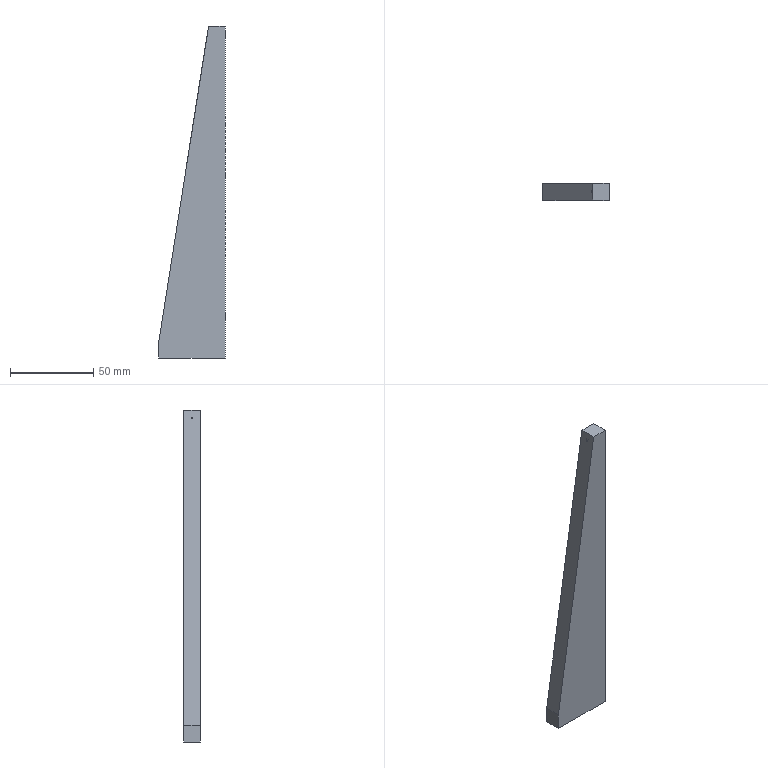Part | SolidWorks | features BaseBody 1 | 1 solid | 27 faces | box 40 x 10 x 200 mm | volume 51054 mm3 | cylinder 10 | cone 10 | plane 7 | commonest cylinder face diameters 3.3 x10
STEP:
#1=CARTESIAN_POINT('',(9.9,0.,96.65));
#2=VERTEX_POINT('',#1);
#3=CARTESIAN_POINT('',(20.,0.,96.65));
#4=VERTEX_POINT('',#3);
#5=CARTESIAN_POINT('',(20.,0.,96.65));
#6=DIRECTION('',(1.,0.,0.));
#7=VECTOR('',#6,1000.);
#8=LINE('',#5,#7);
#9=EDGE_CURVE('',#2,#4,#8,.T.);
#10=ORIENTED_EDGE('',*,*,#9,.F.);
#11=CARTESIAN_POINT('',(9.9,0.,93.35));
#12=VERTEX_POINT('',#11);
#13=CARTESIAN_POINT('',(9.9,0.,95.));
#14=DIRECTION('',(1.,0.,0.));
#15=DIRECTION('',(0.,0.,-1.));
#16=AXIS2_PLACEMENT_3D('',#13,#14,#15);
#17=CIRCLE('',#16,1.65);
#18=EDGE_CURVE('',#12,#2,#17,.T.);
#19=ORIENTED_EDGE('',*,*,#18,.F.);
#20=CARTESIAN_POINT('',(20.,0.,93.35));
#21=VERTEX_POINT('',#20);
#22=CARTESIAN_POINT('',(20.,0.,93.35));
#23=DIRECTION('',(1.,0.,0.));
#24=VECTOR('',#23,1000.);
#25=LINE('',#22,#24);
#26=EDGE_CURVE('',#12,#21,#25,.T.);
#27=ORIENTED_EDGE('',*,*,#26,.T.);
#28=CARTESIAN_POINT('',(20.,0.,95.));
#29=DIRECTION('',(1.,0.,0.));
#30=DIRECTION('',(0.,0.,-1.));
#31=AXIS2_PLACEMENT_3D('',#28,#29,#30);
#32=CIRCLE('',#31,1.65);
#33=EDGE_CURVE('',#21,#4,#32,.T.);
#34=ORIENTED_EDGE('',*,*,#33,.T.);
#35=EDGE_LOOP('',(#10,#19,#27,#34));
#36=FACE_OUTER_BOUND('',#35,.T.);
#37=CARTESIAN_POINT('',(20.,0.,95.));
#38=DIRECTION('',(1.,0.,0.));
#39=DIRECTION('',(0.,0.,-1.));
#40=AXIS2_PLACEMENT_3D('',#37,#38,#39);
#41=CYLINDRICAL_SURFACE('',#40,1.65);
#42=ADVANCED_FACE('',(#36),#41,.F.);
#43=CARTESIAN_POINT('',(9.318,0.,95.682));
#44=VERTEX_POINT('',#43);
#45=CARTESIAN_POINT('',(9.9,0.,96.65));
#46=DIRECTION('',(0.515,0.,0.8572));
#47=VECTOR('',#46,1000.);
#48=LINE('',#45,#47);
#49=EDGE_CURVE('',#44,#2,#48,.T.);
#50=ORIENTED_EDGE('',*,*,#49,.F.);
#51=CARTESIAN_POINT('',(9.148,0.,94.602));
#52=VERTEX_POINT('',#51);
#53=CARTESIAN_POINT('',(9.148,0.,94.602));
#54=CARTESIAN_POINT('',(9.148,1.042,94.602));
#55=CARTESIAN_POINT('',(9.318,1.042,95.682));
#56=CARTESIAN_POINT('',(9.318,0.,95.682));
#57=(BOUNDED_CURVE()B_SPLINE_CURVE(3,(#53,#54,#55,#56),.UNSPECIFIED.,.F.,.F.)B_SPLINE_CURVE_WITH_KNOTS((4,4),(3.142,6.283),.UNSPECIFIED.)CURVE()GEOMETRIC_REPRESENTATION_ITEM()RATIONAL_B_SPLINE_CURVE((1.,0.3333,0.3333,1.))REPRESENTATION_ITEM(''));
#58=EDGE_CURVE('',#52,#44,#57,.T.);
#59=ORIENTED_EDGE('',*,*,#58,.F.);
#60=CARTESIAN_POINT('',(9.9,0.,93.35));
#61=DIRECTION('',(0.515,0.,-0.8572));
#62=VECTOR('',#61,1000.);
#63=LINE('',#60,#62);
#64=EDGE_CURVE('',#52,#12,#63,.T.);
#65=ORIENTED_EDGE('',*,*,#64,.T.);
#66=ORIENTED_EDGE('',*,*,#18,.T.);
#67=EDGE_LOOP('',(#50,#59,#65,#66));
#68=FACE_OUTER_BOUND('',#67,.T.);
#69=CARTESIAN_POINT('',(9.9,0.,95.));
#70=DIRECTION('',(1.,0.,0.));
#71=DIRECTION('',(0.,0.,-1.));
#72=AXIS2_PLACEMENT_3D('',#69,#70,#71);
#73=CONICAL_SURFACE('',#72,1.65,1.03);
#74=ADVANCED_FACE('',(#68),#73,.F.);
#75=CARTESIAN_POINT('',(9.9,0.,11.65));
#76=VERTEX_POINT('',#75);
#77=CARTESIAN_POINT('',(20.,0.,11.65));
#78=VERTEX_POINT('',#77);
#79=CARTESIAN_POINT('',(20.,0.,11.65));
#80=DIRECTION('',(1.,0.,0.));
#81=VECTOR('',#80,1000.);
#82=LINE('',#79,#81);
#83=EDGE_CURVE('',#76,#78,#82,.T.);
#84=ORIENTED_EDGE('',*,*,#83,.F.);
#85=CARTESIAN_POINT('',(9.9,0.,8.35));
#86=VERTEX_POINT('',#85);
#87=CARTESIAN_POINT('',(9.9,0.,10.));
#88=DIRECTION('',(1.,0.,0.));
#89=DIRECTION('',(0.,0.,-1.));
#90=AXIS2_PLACEMENT_3D('',#87,#88,#89);
#91=CIRCLE('',#90,1.65);
#92=EDGE_CURVE('',#86,#76,#91,.T.);
#93=ORIENTED_EDGE('',*,*,#92,.F.);
#94=CARTESIAN_POINT('',(20.,0.,8.35));
#95=VERTEX_POINT('',#94);
#96=CARTESIAN_POINT('',(20.,0.,8.35));
#97=DIRECTION('',(1.,0.,0.));
#98=VECTOR('',#97,1000.);
#99=LINE('',#96,#98);
#100=EDGE_CURVE('',#86,#95,#99,.T.);
#101=ORIENTED_EDGE('',*,*,#100,.T.);
#102=CARTESIAN_POINT('',(20.,0.,10.));
#103=DIRECTION('',(1.,0.,0.));
#104=DIRECTION('',(0.,0.,-1.));
#105=AXIS2_PLACEMENT_3D('',#102,#103,#104);
#106=CIRCLE('',#105,1.65);
#107=EDGE_CURVE('',#95,#78,#106,.T.);
#108=ORIENTED_EDGE('',*,*,#107,.T.);
#109=EDGE_LOOP('',(#84,#93,#101,#108));
#110=FACE_OUTER_BOUND('',#109,.T.);
#111=CARTESIAN_POINT('',(20.,0.,10.));
#112=DIRECTION('',(1.,0.,0.));
#113=DIRECTION('',(0.,0.,-1.));
#114=AXIS2_PLACEMENT_3D('',#111,#112,#113);
#115=CYLINDRICAL_SURFACE('',#114,1.65);
#116=ADVANCED_FACE('',(#110),#115,.F.);
#117=CARTESIAN_POINT('',(8.909,0.,10.));
#118=VERTEX_POINT('',#117);
#119=CARTESIAN_POINT('',(9.9,0.,11.65));
#120=DIRECTION('',(0.515,0.,0.8572));
#121=VECTOR('',#120,1000.);
#122=LINE('',#119,#121);
#123=EDGE_CURVE('',#118,#76,#122,.T.);
#124=ORIENTED_EDGE('',*,*,#123,.F.);
#125=CARTESIAN_POINT('',(9.9,0.,8.35));
#126=DIRECTION('',(0.515,0.,-0.8572));
#127=VECTOR('',#126,1000.);
#128=LINE('',#125,#127);
#129=EDGE_CURVE('',#118,#86,#128,.T.);
#130=ORIENTED_EDGE('',*,*,#129,.T.);
#131=ORIENTED_EDGE('',*,*,#92,.T.);
#132=EDGE_LOOP('',(#124,#130,#131));
#133=FACE_OUTER_BOUND('',#132,.T.);
#134=CARTESIAN_POINT('',(9.9,0.,10.));
#135=DIRECTION('',(1.,0.,0.));
#136=DIRECTION('',(0.,0.,-1.));
#137=AXIS2_PLACEMENT_3D('',#134,#135,#136);
#138=CONICAL_SURFACE('',#137,1.65,1.03);
#139=ADVANCED_FACE('',(#133),#138,.F.);
#140=CARTESIAN_POINT('',(9.9,0.,-73.35));
#141=VERTEX_POINT('',#140);
#142=CARTESIAN_POINT('',(20.,0.,-73.35));
#143=VERTEX_POINT('',#142);
#144=CARTESIAN_POINT('',(20.,0.,-73.35));
#145=DIRECTION('',(1.,0.,0.));
#146=VECTOR('',#145,1000.);
#147=LINE('',#144,#146);
#148=EDGE_CURVE('',#141,#143,#147,.T.);
#149=ORIENTED_EDGE('',*,*,#148,.F.);
#150=CARTESIAN_POINT('',(9.9,0.,-76.65));
#151=VERTEX_POINT('',#150);
#152=CARTESIAN_POINT('',(9.9,0.,-75.));
#153=DIRECTION('',(1.,0.,0.));
#154=DIRECTION('',(0.,0.,-1.));
#155=AXIS2_PLACEMENT_3D('',#152,#153,#154);
#156=CIRCLE('',#155,1.65);
#157=EDGE_CURVE('',#151,#141,#156,.T.);
#158=ORIENTED_EDGE('',*,*,#157,.F.);
#159=CARTESIAN_POINT('',(20.,0.,-76.65));
#160=VERTEX_POINT('',#159);
#161=CARTESIAN_POINT('',(20.,0.,-76.65));
#162=DIRECTION('',(1.,0.,0.));
#163=VECTOR('',#162,1000.);
#164=LINE('',#161,#163);
#165=EDGE_CURVE('',#151,#160,#164,.T.);
#166=ORIENTED_EDGE('',*,*,#165,.T.);
#167=CARTESIAN_POINT('',(20.,0.,-75.));
#168=DIRECTION('',(1.,0.,0.));
#169=DIRECTION('',(0.,0.,-1.));
#170=AXIS2_PLACEMENT_3D('',#167,#168,#169);
#171=CIRCLE('',#170,1.65);
#172=EDGE_CURVE('',#160,#143,#171,.T.);
#173=ORIENTED_EDGE('',*,*,#172,.T.);
#174=EDGE_LOOP('',(#149,#158,#166,#173));
#175=FACE_OUTER_BOUND('',#174,.T.);
#176=CARTESIAN_POINT('',(20.,0.,-75.));
#177=DIRECTION('',(1.,0.,0.));
#178=DIRECTION('',(0.,0.,-1.));
#179=AXIS2_PLACEMENT_3D('',#176,#177,#178);
#180=CYLINDRICAL_SURFACE('',#179,1.65);
#181=ADVANCED_FACE('',(#175),#180,.F.);
#182=CARTESIAN_POINT('',(8.909,0.,-75.));
#183=VERTEX_POINT('',#182);
#184=CARTESIAN_POINT('',(9.9,0.,-73.35));
#185=DIRECTION('',(0.515,0.,0.8572));
#186=VECTOR('',#185,1000.);
#187=LINE('',#184,#186);
#188=EDGE_CURVE('',#183,#141,#187,.T.);
#189=ORIENTED_EDGE('',*,*,#188,.F.);
#190=CARTESIAN_POINT('',(9.9,0.,-76.65));
#191=DIRECTION('',(0.515,0.,-0.8572));
#192=VECTOR('',#191,1000.);
#193=LINE('',#190,#192);
#194=EDGE_CURVE('',#183,#151,#193,.T.);
#195=ORIENTED_EDGE('',*,*,#194,.T.);
#196=ORIENTED_EDGE('',*,*,#157,.T.);
#197=EDGE_LOOP('',(#189,#195,#196));
#198=FACE_OUTER_BOUND('',#197,.T.);
#199=CARTESIAN_POINT('',(9.9,0.,-75.));
#200=DIRECTION('',(1.,0.,0.));
#201=DIRECTION('',(0.,0.,-1.));
#202=AXIS2_PLACEMENT_3D('',#199,#200,#201);
#203=CONICAL_SURFACE('',#202,1.65,1.03);
#204=ADVANCED_FACE('',(#198),#203,.F.);
#205=CARTESIAN_POINT('',(-13.35,0.,-89.9));
#206=VERTEX_POINT('',#205);
#207=CARTESIAN_POINT('',(-13.35,0.,-100.));
#208=VERTEX_POINT('',#207);
#209=CARTESIAN_POINT('',(-13.35,0.,-100.));
#210=DIRECTION('',(0.,0.,-1.));
#211=VECTOR('',#210,1000.);
#212=LINE('',#209,#211);
#213=EDGE_CURVE('',#206,#208,#212,.T.);
#214=ORIENTED_EDGE('',*,*,#213,.F.);
#215=CARTESIAN_POINT('',(-16.65,0.,-89.9));
#216=VERTEX_POINT('',#215);
#217=CARTESIAN_POINT('',(-15.,0.,-89.9));
#218=DIRECTION('',(0.,0.,-1.));
#219=DIRECTION('',(-1.,0.,0.));
#220=AXIS2_PLACEMENT_3D('',#217,#218,#219);
#221=CIRCLE('',#220,1.65);
#222=EDGE_CURVE('',#216,#206,#221,.T.);
#223=ORIENTED_EDGE('',*,*,#222,.F.);
#224=CARTESIAN_POINT('',(-16.65,0.,-100.));
#225=VERTEX_POINT('',#224);
#226=CARTESIAN_POINT('',(-16.65,0.,-100.));
#227=DIRECTION('',(0.,0.,-1.));
#228=VECTOR('',#227,1000.);
#229=LINE('',#226,#228);
#230=EDGE_CURVE('',#216,#225,#229,.T.);
#231=ORIENTED_EDGE('',*,*,#230,.T.);
#232=CARTESIAN_POINT('',(-15.,0.,-100.));
#233=DIRECTION('',(0.,0.,-1.));
#234=DIRECTION('',(-1.,0.,0.));
#235=AXIS2_PLACEMENT_3D('',#232,#233,#234);
#236=CIRCLE('',#235,1.65);
#237=EDGE_CURVE('',#225,#208,#236,.T.);
#238=ORIENTED_EDGE('',*,*,#237,.T.);
#239=EDGE_LOOP('',(#214,#223,#231,#238));
#240=FACE_OUTER_BOUND('',#239,.T.);
#241=CARTESIAN_POINT('',(-15.,0.,-100.));
#242=DIRECTION('',(0.,0.,-1.));
#243=DIRECTION('',(-1.,0.,0.));
#244=AXIS2_PLACEMENT_3D('',#241,#242,#243);
#245=CYLINDRICAL_SURFACE('',#244,1.65);
#246=ADVANCED_FACE('',(#240),#245,.F.);
#247=CARTESIAN_POINT('',(-15.,0.,-88.909));
#248=VERTEX_POINT('',#247);
#249=CARTESIAN_POINT('',(-13.35,0.,-89.9));
#250=DIRECTION('',(0.8572,0.,-0.515));
#251=VECTOR('',#250,1000.);
#252=LINE('',#249,#251);
#253=EDGE_CURVE('',#248,#206,#252,.T.);
#254=ORIENTED_EDGE('',*,*,#253,.F.);
#255=CARTESIAN_POINT('',(-16.65,0.,-89.9));
#256=DIRECTION('',(-0.8572,0.,-0.515));
#257=VECTOR('',#256,1000.);
#258=LINE('',#255,#257);
#259=EDGE_CURVE('',#248,#216,#258,.T.);
#260=ORIENTED_EDGE('',*,*,#259,.T.);
#261=ORIENTED_EDGE('',*,*,#222,.T.);
#262=EDGE_LOOP('',(#254,#260,#261));
#263=FACE_OUTER_BOUND('',#262,.T.);
#264=CARTESIAN_POINT('',(-15.,0.,-89.9));
#265=DIRECTION('',(0.,0.,-1.));
#266=DIRECTION('',(-1.,0.,0.));
#267=AXIS2_PLACEMENT_3D('',#264,#265,#266);
#268=CONICAL_SURFACE('',#267,1.65,1.03);
#269=ADVANCED_FACE('',(#263),#268,.F.);
#270=CARTESIAN_POINT('',(11.65,0.,-89.9));
#271=VERTEX_POINT('',#270);
#272=CARTESIAN_POINT('',(11.65,0.,-100.));
#273=VERTEX_POINT('',#272);
#274=CARTESIAN_POINT('',(11.65,0.,-100.));
#275=DIRECTION('',(0.,0.,-1.));
#276=VECTOR('',#275,1000.);
#277=LINE('',#274,#276);
#278=EDGE_CURVE('',#271,#273,#277,.T.);
#279=ORIENTED_EDGE('',*,*,#278,.F.);
#280=CARTESIAN_POINT('',(8.35,0.,-89.9));
#281=VERTEX_POINT('',#280);
#282=CARTESIAN_POINT('',(10.,0.,-89.9));
#283=DIRECTION('',(0.,0.,-1.));
#284=DIRECTION('',(-1.,0.,0.));
#285=AXIS2_PLACEMENT_3D('',#282,#283,#284);
#286=CIRCLE('',#285,1.65);
#287=EDGE_CURVE('',#281,#271,#286,.T.);
#288=ORIENTED_EDGE('',*,*,#287,.F.);
#289=CARTESIAN_POINT('',(8.35,0.,-100.));
#290=VERTEX_POINT('',#289);
#291=CARTESIAN_POINT('',(8.35,0.,-100.));
#292=DIRECTION('',(0.,0.,-1.));
#293=VECTOR('',#292,1000.);
#294=LINE('',#291,#293);
#295=EDGE_CURVE('',#281,#290,#294,.T.);
#296=ORIENTED_EDGE('',*,*,#295,.T.);
#297=CARTESIAN_POINT('',(10.,0.,-100.));
#298=DIRECTION('',(0.,0.,-1.));
#299=DIRECTION('',(-1.,0.,0.));
#300=AXIS2_PLACEMENT_3D('',#297,#298,#299);
#301=CIRCLE('',#300,1.65);
#302=EDGE_CURVE('',#290,#273,#301,.T.);
#303=ORIENTED_EDGE('',*,*,#302,.T.);
#304=EDGE_LOOP('',(#279,#288,#296,#303));
#305=FACE_OUTER_BOUND('',#304,.T.);
#306=CARTESIAN_POINT('',(10.,0.,-100.));
#307=DIRECTION('',(0.,0.,-1.));
#308=DIRECTION('',(-1.,0.,0.));
#309=AXIS2_PLACEMENT_3D('',#306,#307,#308);
#310=CYLINDRICAL_SURFACE('',#309,1.65);
#311=ADVANCED_FACE('',(#305),#310,.F.);
#312=CARTESIAN_POINT('',(10.,0.,-88.909));
#313=VERTEX_POINT('',#312);
#314=CARTESIAN_POINT('',(11.65,0.,-89.9));
#315=DIRECTION('',(0.8572,0.,-0.515));
#316=VECTOR('',#315,1000.);
#317=LINE('',#314,#316);
#318=EDGE_CURVE('',#313,#271,#317,.T.);
#319=ORIENTED_EDGE('',*,*,#318,.F.);
#320=CARTESIAN_POINT('',(8.35,0.,-89.9));
#321=DIRECTION('',(-0.8572,0.,-0.515));
#322=VECTOR('',#321,1000.);
#323=LINE('',#320,#322);
#324=EDGE_CURVE('',#313,#281,#323,.T.);
#325=ORIENTED_EDGE('',*,*,#324,.T.);
#326=ORIENTED_EDGE('',*,*,#287,.T.);
#327=EDGE_LOOP('',(#319,#325,#326));
#328=FACE_OUTER_BOUND('',#327,.T.);
#329=CARTESIAN_POINT('',(10.,0.,-89.9));
#330=DIRECTION('',(0.,0.,-1.));
#331=DIRECTION('',(-1.,0.,0.));
#332=AXIS2_PLACEMENT_3D('',#329,#330,#331);
#333=CONICAL_SURFACE('',#332,1.65,1.03);
#334=ADVANCED_FACE('',(#328),#333,.F.);
#335=ORIENTED_EDGE('',*,*,#58,.T.);
#336=CARTESIAN_POINT('',(9.318,0.,95.682));
#337=CARTESIAN_POINT('',(9.318,-1.042,95.682));
#338=CARTESIAN_POINT('',(9.148,-1.042,94.602));
#339=CARTESIAN_POINT('',(9.148,0.,94.602));
#340=(BOUNDED_CURVE()B_SPLINE_CURVE(3,(#336,#337,#338,#339),.UNSPECIFIED.,.F.,.F.)B_SPLINE_CURVE_WITH_KNOTS((4,4),(0.,3.142),.UNSPECIFIED.)CURVE()GEOMETRIC_REPRESENTATION_ITEM()RATIONAL_B_SPLINE_CURVE((1.,0.3333,0.3333,1.))REPRESENTATION_ITEM(''));
#341=EDGE_CURVE('',#44,#52,#340,.T.);
#342=ORIENTED_EDGE('',*,*,#341,.T.);
#343=EDGE_LOOP('',(#335,#342));
#344=FACE_BOUND('',#343,.T.);
#345=CARTESIAN_POINT('',(10.,-5.,100.));
#346=VERTEX_POINT('',#345);
#347=CARTESIAN_POINT('',(10.,5.,100.));
#348=VERTEX_POINT('',#347);
#349=CARTESIAN_POINT('',(10.,-197.354,100.));
#350=DIRECTION('',(0.,1.,0.));
#351=VECTOR('',#350,1000.);
#352=LINE('',#349,#351);
#353=EDGE_CURVE('',#346,#348,#352,.T.);
#354=ORIENTED_EDGE('',*,*,#353,.T.);
#355=CARTESIAN_POINT('',(-20.,5.,-90.));
#356=VERTEX_POINT('',#355);
#357=CARTESIAN_POINT('',(10.,5.,100.));
#358=DIRECTION('',(-0.156,0.,-0.9878));
#359=VECTOR('',#358,1000.);
#360=LINE('',#357,#359);
#361=EDGE_CURVE('',#348,#356,#360,.T.);
#362=ORIENTED_EDGE('',*,*,#361,.T.);
#363=CARTESIAN_POINT('',(-20.,-5.,-90.));
#364=VERTEX_POINT('',#363);
#365=CARTESIAN_POINT('',(-20.,-197.354,-90.));
#366=DIRECTION('',(0.,1.,0.));
#367=VECTOR('',#366,1000.);
#368=LINE('',#365,#367);
#369=EDGE_CURVE('',#364,#356,#368,.T.);
#370=ORIENTED_EDGE('',*,*,#369,.F.);
#371=CARTESIAN_POINT('',(10.,-5.,100.));
#372=DIRECTION('',(-0.156,0.,-0.9878));
#373=VECTOR('',#372,1000.);
#374=LINE('',#371,#373);
#375=EDGE_CURVE('',#346,#364,#374,.T.);
#376=ORIENTED_EDGE('',*,*,#375,.F.);
#377=EDGE_LOOP('',(#354,#362,#370,#376));
#378=FACE_OUTER_BOUND('',#377,.T.);
#379=CARTESIAN_POINT('',(10.,-197.354,100.));
#380=DIRECTION('',(0.9878,0.,-0.156));
#381=DIRECTION('',(0.,-1.,0.));
#382=AXIS2_PLACEMENT_3D('',#379,#380,#381);
#383=PLANE('',#382);
#384=ADVANCED_FACE('',(#344,#378),#383,.F.);
#385=ORIENTED_EDGE('',*,*,#375,.T.);
#386=CARTESIAN_POINT('',(-20.,-5.,-100.));
#387=VERTEX_POINT('',#386);
#388=CARTESIAN_POINT('',(-20.,-5.,100.));
#389=DIRECTION('',(0.,0.,1.));
#390=VECTOR('',#389,1000.);
#391=LINE('',#388,#390);
#392=EDGE_CURVE('',#387,#364,#391,.T.);
#393=ORIENTED_EDGE('',*,*,#392,.F.);
#394=CARTESIAN_POINT('',(20.,-5.,-100.));
#395=VERTEX_POINT('',#394);
#396=CARTESIAN_POINT('',(-20.,-5.,-100.));
#397=DIRECTION('',(-1.,0.,0.));
#398=VECTOR('',#397,1000.);
#399=LINE('',#396,#398);
#400=EDGE_CURVE('',#395,#387,#399,.T.);
#401=ORIENTED_EDGE('',*,*,#400,.F.);
#402=CARTESIAN_POINT('',(20.,-5.,100.));
#403=VERTEX_POINT('',#402);
#404=CARTESIAN_POINT('',(20.,-5.,100.));
#405=DIRECTION('',(0.,0.,-1.));
#406=VECTOR('',#405,1000.);
#407=LINE('',#404,#406);
#408=EDGE_CURVE('',#403,#395,#407,.T.);
#409=ORIENTED_EDGE('',*,*,#408,.F.);
#410=CARTESIAN_POINT('',(-20.,-5.,100.));
#411=DIRECTION('',(1.,0.,0.));
#412=VECTOR('',#411,1000.);
#413=LINE('',#410,#412);
#414=EDGE_CURVE('',#346,#403,#413,.T.);
#415=ORIENTED_EDGE('',*,*,#414,.F.);
#416=EDGE_LOOP('',(#385,#393,#401,#409,#415));
#417=FACE_OUTER_BOUND('',#416,.T.);
#418=CARTESIAN_POINT('',(0.,-5.,0.));
#419=DIRECTION('',(0.,-1.,0.));
#420=DIRECTION('',(0.,0.,-1.));
#421=AXIS2_PLACEMENT_3D('',#418,#419,#420);
#422=PLANE('',#421);
#423=ADVANCED_FACE('',(#417),#422,.T.);
#424=CARTESIAN_POINT('',(-20.,5.,-100.));
#425=VERTEX_POINT('',#424);
#426=CARTESIAN_POINT('',(-20.,5.,100.));
#427=DIRECTION('',(0.,0.,1.));
#428=VECTOR('',#427,1000.);
#429=LINE('',#426,#428);
#430=EDGE_CURVE('',#425,#356,#429,.T.);
#431=ORIENTED_EDGE('',*,*,#430,.T.);
#432=ORIENTED_EDGE('',*,*,#361,.F.);
#433=CARTESIAN_POINT('',(20.,5.,100.));
#434=VERTEX_POINT('',#433);
#435=CARTESIAN_POINT('',(-20.,5.,100.));
#436=DIRECTION('',(1.,0.,0.));
#437=VECTOR('',#436,1000.);
#438=LINE('',#435,#437);
#439=EDGE_CURVE('',#348,#434,#438,.T.);
#440=ORIENTED_EDGE('',*,*,#439,.T.);
#441=CARTESIAN_POINT('',(20.,5.,-100.));
#442=VERTEX_POINT('',#441);
#443=CARTESIAN_POINT('',(20.,5.,100.));
#444=DIRECTION('',(0.,0.,-1.));
#445=VECTOR('',#444,1000.);
#446=LINE('',#443,#445);
#447=EDGE_CURVE('',#434,#442,#446,.T.);
#448=ORIENTED_EDGE('',*,*,#447,.T.);
#449=CARTESIAN_POINT('',(-20.,5.,-100.));
#450=DIRECTION('',(-1.,0.,0.));
#451=VECTOR('',#450,1000.);
#452=LINE('',#449,#451);
#453=EDGE_CURVE('',#442,#425,#452,.T.);
#454=ORIENTED_EDGE('',*,*,#453,.T.);
#455=EDGE_LOOP('',(#431,#432,#440,#448,#454));
#456=FACE_OUTER_BOUND('',#455,.T.);
#457=CARTESIAN_POINT('',(0.,5.,0.));
#458=DIRECTION('',(0.,-1.,0.));
#459=DIRECTION('',(0.,0.,-1.));
#460=AXIS2_PLACEMENT_3D('',#457,#458,#459);
#461=PLANE('',#460);
#462=ADVANCED_FACE('',(#456),#461,.F.);
#463=ORIENTED_EDGE('',*,*,#439,.F.);
#464=ORIENTED_EDGE('',*,*,#353,.F.);
#465=ORIENTED_EDGE('',*,*,#414,.T.);
#466=CARTESIAN_POINT('',(20.,5.,100.));
#467=DIRECTION('',(0.,-1.,0.));
#468=VECTOR('',#467,1000.);
#469=LINE('',#466,#468);
#470=EDGE_CURVE('',#434,#403,#469,.T.);
#471=ORIENTED_EDGE('',*,*,#470,.F.);
#472=EDGE_LOOP('',(#463,#464,#465,#471));
#473=FACE_OUTER_BOUND('',#472,.T.);
#474=CARTESIAN_POINT('',(-20.,5.,100.));
#475=DIRECTION('',(0.,0.,-1.));
#476=DIRECTION('',(0.,-1.,0.));
#477=AXIS2_PLACEMENT_3D('',#474,#475,#476);
#478=PLANE('',#477);
#479=ADVANCED_FACE('',(#473),#478,.F.);
#480=ORIENTED_EDGE('',*,*,#392,.T.);
#481=ORIENTED_EDGE('',*,*,#369,.T.);
#482=ORIENTED_EDGE('',*,*,#430,.F.);
#483=CARTESIAN_POINT('',(-20.,5.,-100.));
#484=DIRECTION('',(0.,-1.,0.));
#485=VECTOR('',#484,1000.);
#486=LINE('',#483,#485);
#487=EDGE_CURVE('',#425,#387,#486,.T.);
#488=ORIENTED_EDGE('',*,*,#487,.T.);
#489=EDGE_LOOP('',(#480,#481,#482,#488));
#490=FACE_OUTER_BOUND('',#489,.T.);
#491=CARTESIAN_POINT('',(-20.,5.,100.));
#492=DIRECTION('',(1.,0.,0.));
#493=DIRECTION('',(0.,1.,0.));
#494=AXIS2_PLACEMENT_3D('',#491,#492,#493);
#495=PLANE('',#494);
#496=ADVANCED_FACE('',(#490),#495,.F.);
#497=ORIENTED_EDGE('',*,*,#302,.F.);
#498=CARTESIAN_POINT('',(10.,0.,-100.));
#499=DIRECTION('',(0.,0.,-1.));
#500=DIRECTION('',(-1.,0.,0.));
#501=AXIS2_PLACEMENT_3D('',#498,#499,#500);
#502=CIRCLE('',#501,1.65);
#503=EDGE_CURVE('',#273,#290,#502,.T.);
#504=ORIENTED_EDGE('',*,*,#503,.F.);
#505=EDGE_LOOP('',(#497,#504));
#506=FACE_BOUND('',#505,.T.);
#507=ORIENTED_EDGE('',*,*,#237,.F.);
#508=CARTESIAN_POINT('',(-15.,0.,-100.));
#509=DIRECTION('',(0.,0.,-1.));
#510=DIRECTION('',(-1.,0.,0.));
#511=AXIS2_PLACEMENT_3D('',#508,#509,#510);
#512=CIRCLE('',#511,1.65);
#513=EDGE_CURVE('',#208,#225,#512,.T.);
#514=ORIENTED_EDGE('',*,*,#513,.F.);
#515=EDGE_LOOP('',(#507,#514));
#516=FACE_BOUND('',#515,.T.);
#517=ORIENTED_EDGE('',*,*,#400,.T.);
#518=ORIENTED_EDGE('',*,*,#487,.F.);
#519=ORIENTED_EDGE('',*,*,#453,.F.);
#520=CARTESIAN_POINT('',(20.,5.,-100.));
#521=DIRECTION('',(0.,-1.,0.));
#522=VECTOR('',#521,1000.);
#523=LINE('',#520,#522);
#524=EDGE_CURVE('',#442,#395,#523,.T.);
#525=ORIENTED_EDGE('',*,*,#524,.T.);
#526=EDGE_LOOP('',(#517,#518,#519,#525));
#527=FACE_OUTER_BOUND('',#526,.T.);
#528=CARTESIAN_POINT('',(-20.,5.,-100.));
#529=DIRECTION('',(0.,0.,1.));
#530=DIRECTION('',(1.,0.,0.));
#531=AXIS2_PLACEMENT_3D('',#528,#529,#530);
#532=PLANE('',#531);
#533=ADVANCED_FACE('',(#506,#516,#527),#532,.F.);
#534=ORIENTED_EDGE('',*,*,#172,.F.);
#535=CARTESIAN_POINT('',(20.,0.,-75.));
#536=DIRECTION('',(1.,0.,0.));
#537=DIRECTION('',(0.,0.,-1.));
#538=AXIS2_PLACEMENT_3D('',#535,#536,#537);
#539=CIRCLE('',#538,1.65);
#540=EDGE_CURVE('',#143,#160,#539,.T.);
#541=ORIENTED_EDGE('',*,*,#540,.F.);
#542=EDGE_LOOP('',(#534,#541));
#543=FACE_BOUND('',#542,.T.);
#544=ORIENTED_EDGE('',*,*,#107,.F.);
#545=CARTESIAN_POINT('',(20.,0.,10.));
#546=DIRECTION('',(1.,0.,0.));
#547=DIRECTION('',(0.,0.,-1.));
#548=AXIS2_PLACEMENT_3D('',#545,#546,#547);
#549=CIRCLE('',#548,1.65);
#550=EDGE_CURVE('',#78,#95,#549,.T.);
#551=ORIENTED_EDGE('',*,*,#550,.F.);
#552=EDGE_LOOP('',(#544,#551));
#553=FACE_BOUND('',#552,.T.);
#554=ORIENTED_EDGE('',*,*,#33,.F.);
#555=CARTESIAN_POINT('',(20.,0.,95.));
#556=DIRECTION('',(1.,0.,0.));
#557=DIRECTION('',(0.,0.,-1.));
#558=AXIS2_PLACEMENT_3D('',#555,#556,#557);
#559=CIRCLE('',#558,1.65);
#560=EDGE_CURVE('',#4,#21,#559,.T.);
#561=ORIENTED_EDGE('',*,*,#560,.F.);
#562=EDGE_LOOP('',(#554,#561));
#563=FACE_BOUND('',#562,.T.);
#564=ORIENTED_EDGE('',*,*,#408,.T.);
#565=ORIENTED_EDGE('',*,*,#524,.F.);
#566=ORIENTED_EDGE('',*,*,#447,.F.);
#567=ORIENTED_EDGE('',*,*,#470,.T.);
#568=EDGE_LOOP('',(#564,#565,#566,#567));
#569=FACE_OUTER_BOUND('',#568,.T.);
#570=CARTESIAN_POINT('',(20.,5.,100.));
#571=DIRECTION('',(-1.,0.,0.));
#572=DIRECTION('',(0.,0.,1.));
#573=AXIS2_PLACEMENT_3D('',#570,#571,#572);
#574=PLANE('',#573);
#575=ADVANCED_FACE('',(#543,#553,#563,#569),#574,.F.);
#576=ORIENTED_EDGE('',*,*,#324,.F.);
#577=ORIENTED_EDGE('',*,*,#318,.T.);
#578=CARTESIAN_POINT('',(10.,0.,-89.9));
#579=DIRECTION('',(0.,0.,-1.));
#580=DIRECTION('',(-1.,0.,0.));
#581=AXIS2_PLACEMENT_3D('',#578,#579,#580);
#582=CIRCLE('',#581,1.65);
#583=EDGE_CURVE('',#271,#281,#582,.T.);
#584=ORIENTED_EDGE('',*,*,#583,.T.);
#585=EDGE_LOOP('',(#576,#577,#584));
#586=FACE_OUTER_BOUND('',#585,.T.);
#587=CARTESIAN_POINT('',(10.,0.,-89.9));
#588=DIRECTION('',(0.,0.,-1.));
#589=DIRECTION('',(-1.,0.,0.));
#590=AXIS2_PLACEMENT_3D('',#587,#588,#589);
#591=CONICAL_SURFACE('',#590,1.65,1.03);
#592=ADVANCED_FACE('',(#586),#591,.F.);
#593=ORIENTED_EDGE('',*,*,#583,.F.);
#594=ORIENTED_EDGE('',*,*,#278,.T.);
#595=ORIENTED_EDGE('',*,*,#503,.T.);
#596=ORIENTED_EDGE('',*,*,#295,.F.);
#597=EDGE_LOOP('',(#593,#594,#595,#596));
#598=FACE_OUTER_BOUND('',#597,.T.);
#599=CARTESIAN_POINT('',(10.,0.,-100.));
#600=DIRECTION('',(0.,0.,-1.));
#601=DIRECTION('',(-1.,0.,0.));
#602=AXIS2_PLACEMENT_3D('',#599,#600,#601);
#603=CYLINDRICAL_SURFACE('',#602,1.65);
#604=ADVANCED_FACE('',(#598),#603,.F.);
#605=ORIENTED_EDGE('',*,*,#259,.F.);
#606=ORIENTED_EDGE('',*,*,#253,.T.);
#607=CARTESIAN_POINT('',(-15.,0.,-89.9));
#608=DIRECTION('',(0.,0.,-1.));
#609=DIRECTION('',(-1.,0.,0.));
#610=AXIS2_PLACEMENT_3D('',#607,#608,#609);
#611=CIRCLE('',#610,1.65);
#612=EDGE_CURVE('',#206,#216,#611,.T.);
#613=ORIENTED_EDGE('',*,*,#612,.T.);
#614=EDGE_LOOP('',(#605,#606,#613));
#615=FACE_OUTER_BOUND('',#614,.T.);
#616=CARTESIAN_POINT('',(-15.,0.,-89.9));
#617=DIRECTION('',(0.,0.,-1.));
#618=DIRECTION('',(-1.,0.,0.));
#619=AXIS2_PLACEMENT_3D('',#616,#617,#618);
#620=CONICAL_SURFACE('',#619,1.65,1.03);
#621=ADVANCED_FACE('',(#615),#620,.F.);
#622=ORIENTED_EDGE('',*,*,#612,.F.);
#623=ORIENTED_EDGE('',*,*,#213,.T.);
#624=ORIENTED_EDGE('',*,*,#513,.T.);
#625=ORIENTED_EDGE('',*,*,#230,.F.);
#626=EDGE_LOOP('',(#622,#623,#624,#625));
#627=FACE_OUTER_BOUND('',#626,.T.);
#628=CARTESIAN_POINT('',(-15.,0.,-100.));
#629=DIRECTION('',(0.,0.,-1.));
#630=DIRECTION('',(-1.,0.,0.));
#631=AXIS2_PLACEMENT_3D('',#628,#629,#630);
#632=CYLINDRICAL_SURFACE('',#631,1.65);
#633=ADVANCED_FACE('',(#627),#632,.F.);
#634=ORIENTED_EDGE('',*,*,#194,.F.);
#635=ORIENTED_EDGE('',*,*,#188,.T.);
#636=CARTESIAN_POINT('',(9.9,0.,-75.));
#637=DIRECTION('',(1.,0.,0.));
#638=DIRECTION('',(0.,0.,-1.));
#639=AXIS2_PLACEMENT_3D('',#636,#637,#638);
#640=CIRCLE('',#639,1.65);
#641=EDGE_CURVE('',#141,#151,#640,.T.);
#642=ORIENTED_EDGE('',*,*,#641,.T.);
#643=EDGE_LOOP('',(#634,#635,#642));
#644=FACE_OUTER_BOUND('',#643,.T.);
#645=CARTESIAN_POINT('',(9.9,0.,-75.));
#646=DIRECTION('',(1.,0.,0.));
#647=DIRECTION('',(0.,0.,-1.));
#648=AXIS2_PLACEMENT_3D('',#645,#646,#647);
#649=CONICAL_SURFACE('',#648,1.65,1.03);
#650=ADVANCED_FACE('',(#644),#649,.F.);
#651=ORIENTED_EDGE('',*,*,#641,.F.);
#652=ORIENTED_EDGE('',*,*,#148,.T.);
#653=ORIENTED_EDGE('',*,*,#540,.T.);
#654=ORIENTED_EDGE('',*,*,#165,.F.);
#655=EDGE_LOOP('',(#651,#652,#653,#654));
#656=FACE_OUTER_BOUND('',#655,.T.);
#657=CARTESIAN_POINT('',(20.,0.,-75.));
#658=DIRECTION('',(1.,0.,0.));
#659=DIRECTION('',(0.,0.,-1.));
#660=AXIS2_PLACEMENT_3D('',#657,#658,#659);
#661=CYLINDRICAL_SURFACE('',#660,1.65);
#662=ADVANCED_FACE('',(#656),#661,.F.);
#663=ORIENTED_EDGE('',*,*,#129,.F.);
#664=ORIENTED_EDGE('',*,*,#123,.T.);
#665=CARTESIAN_POINT('',(9.9,0.,10.));
#666=DIRECTION('',(1.,0.,0.));
#667=DIRECTION('',(0.,0.,-1.));
#668=AXIS2_PLACEMENT_3D('',#665,#666,#667);
#669=CIRCLE('',#668,1.65);
#670=EDGE_CURVE('',#76,#86,#669,.T.);
#671=ORIENTED_EDGE('',*,*,#670,.T.);
#672=EDGE_LOOP('',(#663,#664,#671));
#673=FACE_OUTER_BOUND('',#672,.T.);
#674=CARTESIAN_POINT('',(9.9,0.,10.));
#675=DIRECTION('',(1.,0.,0.));
#676=DIRECTION('',(0.,0.,-1.));
#677=AXIS2_PLACEMENT_3D('',#674,#675,#676);
#678=CONICAL_SURFACE('',#677,1.65,1.03);
#679=ADVANCED_FACE('',(#673),#678,.F.);
#680=ORIENTED_EDGE('',*,*,#670,.F.);
#681=ORIENTED_EDGE('',*,*,#83,.T.);
#682=ORIENTED_EDGE('',*,*,#550,.T.);
#683=ORIENTED_EDGE('',*,*,#100,.F.);
#684=EDGE_LOOP('',(#680,#681,#682,#683));
#685=FACE_OUTER_BOUND('',#684,.T.);
#686=CARTESIAN_POINT('',(20.,0.,10.));
#687=DIRECTION('',(1.,0.,0.));
#688=DIRECTION('',(0.,0.,-1.));
#689=AXIS2_PLACEMENT_3D('',#686,#687,#688);
#690=CYLINDRICAL_SURFACE('',#689,1.65);
#691=ADVANCED_FACE('',(#685),#690,.F.);
#692=ORIENTED_EDGE('',*,*,#341,.F.);
#693=ORIENTED_EDGE('',*,*,#49,.T.);
#694=CARTESIAN_POINT('',(9.9,0.,95.));
#695=DIRECTION('',(1.,0.,0.));
#696=DIRECTION('',(0.,0.,-1.));
#697=AXIS2_PLACEMENT_3D('',#694,#695,#696);
#698=CIRCLE('',#697,1.65);
#699=EDGE_CURVE('',#2,#12,#698,.T.);
#700=ORIENTED_EDGE('',*,*,#699,.T.);
#701=ORIENTED_EDGE('',*,*,#64,.F.);
#702=EDGE_LOOP('',(#692,#693,#700,#701));
#703=FACE_OUTER_BOUND('',#702,.T.);
#704=CARTESIAN_POINT('',(9.9,0.,95.));
#705=DIRECTION('',(1.,0.,0.));
#706=DIRECTION('',(0.,0.,-1.));
#707=AXIS2_PLACEMENT_3D('',#704,#705,#706);
#708=CONICAL_SURFACE('',#707,1.65,1.03);
#709=ADVANCED_FACE('',(#703),#708,.F.);
#710=ORIENTED_EDGE('',*,*,#699,.F.);
#711=ORIENTED_EDGE('',*,*,#9,.T.);
#712=ORIENTED_EDGE('',*,*,#560,.T.);
#713=ORIENTED_EDGE('',*,*,#26,.F.);
#714=EDGE_LOOP('',(#710,#711,#712,#713));
#715=FACE_OUTER_BOUND('',#714,.T.);
#716=CARTESIAN_POINT('',(20.,0.,95.));
#717=DIRECTION('',(1.,0.,0.));
#718=DIRECTION('',(0.,0.,-1.));
#719=AXIS2_PLACEMENT_3D('',#716,#717,#718);
#720=CYLINDRICAL_SURFACE('',#719,1.65);
#721=ADVANCED_FACE('',(#715),#720,.F.);
#722=CLOSED_SHELL('',(#42,#74,#116,#139,#181,#204,#246,#269,#311,#334,#384,#423,#462,#479,#496,#533,#575,#592,#604,#621,#633,#650,#662,#679,#691,#709,#721));
#723=MANIFOLD_SOLID_BREP('',#722);
#724=CARTESIAN_POINT('',(0.,0.,0.));
#725=DIRECTION('',(0.,0.,1.));
#726=DIRECTION('',(1.,0.,0.));
#727=AXIS2_PLACEMENT_3D('',#724,#725,#726);
#728=(LENGTH_UNIT()NAMED_UNIT(*)SI_UNIT(.MILLI.,.METRE.));
#729=UNCERTAINTY_MEASURE_WITH_UNIT(LENGTH_MEASURE(0.00001),#728,'','');
#730=(NAMED_UNIT(*)PLANE_ANGLE_UNIT()SI_UNIT($,.RADIAN.));
#731=(NAMED_UNIT(*)SI_UNIT($,.STERADIAN.)SOLID_ANGLE_UNIT());
#732=(GEOMETRIC_REPRESENTATION_CONTEXT(3)GLOBAL_UNCERTAINTY_ASSIGNED_CONTEXT((#729))GLOBAL_UNIT_ASSIGNED_CONTEXT((#728,#730,#731))REPRESENTATION_CONTEXT('',''));
#733=ADVANCED_BREP_SHAPE_REPRESENTATION('',(#723,#727),#732);